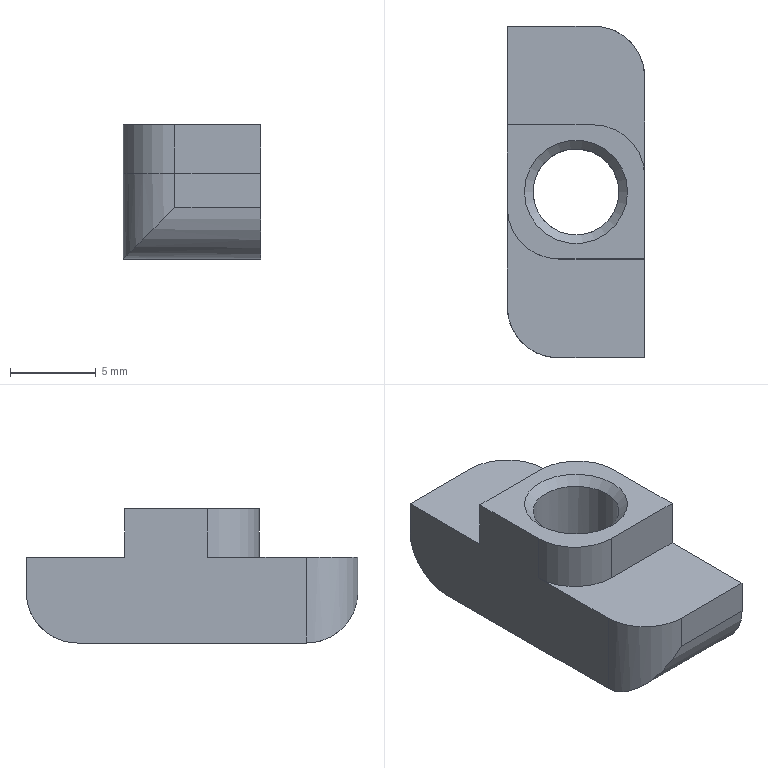Part | NX | features DATUM_CSYS 4, SKETCH 3, EXTRUDE 2, BLEND 1, HOLE PACKAGE 1, SIMPLE HOLE 1, SYMBOLIC_THREAD 1 | 1 solid | 19 faces | box 8 x 19.3 x 7.8 mm | volume 733.523 mm3 | plane 10 | cylinder 7 | cone 2 | commonest cylinder face diameters 6 x6 5 x1
STEP:
#1=CARTESIAN_POINT('',(1.,3.9,0.));
#2=VERTEX_POINT('',#1);
#3=CARTESIAN_POINT('',(-4.,3.9,0.));
#4=VERTEX_POINT('',#3);
#5=CARTESIAN_POINT('',(1.,3.9,0.));
#6=DIRECTION('',(-1.,0.,0.));
#7=VECTOR('',#6,1000.);
#8=LINE('',#5,#7);
#9=EDGE_CURVE('',#2,#4,#8,.T.);
#10=ORIENTED_EDGE('',*,*,#9,.F.);
#11=CARTESIAN_POINT('',(4.,0.9,0.));
#12=VERTEX_POINT('',#11);
#13=CARTESIAN_POINT('',(1.,0.9,0.));
#14=DIRECTION('',(0.,0.,1.));
#15=DIRECTION('',(1.,0.,0.));
#16=AXIS2_PLACEMENT_3D('',#13,#14,#15);
#17=CIRCLE('',#16,3.);
#18=EDGE_CURVE('',#12,#2,#17,.T.);
#19=ORIENTED_EDGE('',*,*,#18,.F.);
#20=CARTESIAN_POINT('',(4.,6.65,0.));
#21=VERTEX_POINT('',#20);
#22=CARTESIAN_POINT('',(4.,0.,0.));
#23=DIRECTION('',(0.,-1.,0.));
#24=VECTOR('',#23,1000.);
#25=LINE('',#22,#24);
#26=EDGE_CURVE('',#21,#12,#25,.T.);
#27=ORIENTED_EDGE('',*,*,#26,.F.);
#28=CARTESIAN_POINT('',(1.,9.65,0.));
#29=VERTEX_POINT('',#28);
#30=CARTESIAN_POINT('',(1.,6.65,0.));
#31=DIRECTION('',(0.,0.,-1.));
#32=DIRECTION('',(0.,1.,0.));
#33=AXIS2_PLACEMENT_3D('',#30,#31,#32);
#34=CIRCLE('',#33,3.);
#35=EDGE_CURVE('',#21,#29,#34,.F.);
#36=ORIENTED_EDGE('',*,*,#35,.T.);
#37=CARTESIAN_POINT('',(-4.,9.65,0.));
#38=VERTEX_POINT('',#37);
#39=CARTESIAN_POINT('',(4.,9.65,0.));
#40=DIRECTION('',(-1.,0.,0.));
#41=VECTOR('',#40,1000.);
#42=LINE('',#39,#41);
#43=EDGE_CURVE('',#29,#38,#42,.T.);
#44=ORIENTED_EDGE('',*,*,#43,.T.);
#45=CARTESIAN_POINT('',(-4.,9.65,0.));
#46=DIRECTION('',(0.,-1.,0.));
#47=VECTOR('',#46,1000.);
#48=LINE('',#45,#47);
#49=EDGE_CURVE('',#38,#4,#48,.T.);
#50=ORIENTED_EDGE('',*,*,#49,.T.);
#51=EDGE_LOOP('',(#10,#19,#27,#36,#44,#50));
#52=FACE_BOUND('',#51,.T.);
#53=CARTESIAN_POINT('',(4.,9.65,0.));
#54=DIRECTION('',(0.,0.,-1.));
#55=DIRECTION('',(0.,1.,0.));
#56=AXIS2_PLACEMENT_3D('',#53,#54,#55);
#57=PLANE('',#56);
#58=ADVANCED_FACE('',(#52),#57,.F.);
#59=CARTESIAN_POINT('',(4.,-9.65,0.));
#60=VERTEX_POINT('',#59);
#61=CARTESIAN_POINT('',(-1.,-9.65,0.));
#62=VERTEX_POINT('',#61);
#63=CARTESIAN_POINT('',(4.,-9.65,0.));
#64=DIRECTION('',(-1.,0.,0.));
#65=VECTOR('',#64,1000.);
#66=LINE('',#63,#65);
#67=EDGE_CURVE('',#60,#62,#66,.T.);
#68=ORIENTED_EDGE('',*,*,#67,.T.);
#69=CARTESIAN_POINT('',(-1.,-9.65,-2.));
#70=VERTEX_POINT('',#69);
#71=CARTESIAN_POINT('',(-1.,-9.65,0.));
#72=DIRECTION('',(0.,0.,-1.));
#73=VECTOR('',#72,1000.);
#74=LINE('',#71,#73);
#75=EDGE_CURVE('',#62,#70,#74,.T.);
#76=ORIENTED_EDGE('',*,*,#75,.T.);
#77=CARTESIAN_POINT('',(4.,-9.65,-2.));
#78=VERTEX_POINT('',#77);
#79=CARTESIAN_POINT('',(4.,-9.65,-2.));
#80=DIRECTION('',(-1.,0.,0.));
#81=VECTOR('',#80,1000.);
#82=LINE('',#79,#81);
#83=EDGE_CURVE('',#78,#70,#82,.T.);
#84=ORIENTED_EDGE('',*,*,#83,.F.);
#85=CARTESIAN_POINT('',(4.,-9.65,0.));
#86=DIRECTION('',(0.,0.,-1.));
#87=VECTOR('',#86,1000.);
#88=LINE('',#85,#87);
#89=EDGE_CURVE('',#60,#78,#88,.T.);
#90=ORIENTED_EDGE('',*,*,#89,.F.);
#91=EDGE_LOOP('',(#68,#76,#84,#90));
#92=FACE_BOUND('',#91,.T.);
#93=CARTESIAN_POINT('',(4.,-9.65,0.));
#94=DIRECTION('',(0.,1.,0.));
#95=DIRECTION('',(0.,0.,1.));
#96=AXIS2_PLACEMENT_3D('',#93,#94,#95);
#97=PLANE('',#96);
#98=ADVANCED_FACE('',(#92),#97,.F.);
#99=ORIENTED_EDGE('',*,*,#83,.T.);
#100=CARTESIAN_POINT('',(-4.,-6.65,-5.));
#101=VERTEX_POINT('',#100);
#102=CARTESIAN_POINT('',(-1.,-6.65,-2.));
#103=DIRECTION('',(0.7071,0.,-0.7071));
#104=DIRECTION('',(-0.7071,0.,-0.7071));
#105=AXIS2_PLACEMENT_3D('',#102,#103,#104);
#106=ELLIPSE('',#105,4.243,3.);
#107=EDGE_CURVE('',#70,#101,#106,.T.);
#108=ORIENTED_EDGE('',*,*,#107,.T.);
#109=CARTESIAN_POINT('',(4.,-6.65,-5.));
#110=VERTEX_POINT('',#109);
#111=CARTESIAN_POINT('',(4.,-6.65,-5.));
#112=DIRECTION('',(-1.,0.,0.));
#113=VECTOR('',#112,1000.);
#114=LINE('',#111,#113);
#115=EDGE_CURVE('',#110,#101,#114,.T.);
#116=ORIENTED_EDGE('',*,*,#115,.F.);
#117=CARTESIAN_POINT('',(4.,-6.65,-2.));
#118=DIRECTION('',(1.,0.,0.));
#119=DIRECTION('',(0.,1.,0.));
#120=AXIS2_PLACEMENT_3D('',#117,#118,#119);
#121=CIRCLE('',#120,3.);
#122=EDGE_CURVE('',#78,#110,#121,.T.);
#123=ORIENTED_EDGE('',*,*,#122,.F.);
#124=EDGE_LOOP('',(#99,#108,#116,#123));
#125=FACE_BOUND('',#124,.T.);
#126=CARTESIAN_POINT('',(4.,-6.65,-2.));
#127=DIRECTION('',(-1.,0.,0.));
#128=DIRECTION('',(0.,0.,1.));
#129=AXIS2_PLACEMENT_3D('',#126,#127,#128);
#130=CYLINDRICAL_SURFACE('',#129,3.);
#131=ADVANCED_FACE('',(#125),#130,.T.);
#132=CARTESIAN_POINT('',(0.,-3.,-5.));
#133=VERTEX_POINT('',#132);
#134=CARTESIAN_POINT('',(0.,0.,-5.));
#135=DIRECTION('',(0.,0.,1.));
#136=DIRECTION('',(0.,-1.,0.));
#137=AXIS2_PLACEMENT_3D('',#134,#135,#136);
#138=CIRCLE('',#137,3.);
#139=EDGE_CURVE('',#133,#133,#138,.T.);
#140=ORIENTED_EDGE('',*,*,#139,.T.);
#141=EDGE_LOOP('',(#140));
#142=FACE_BOUND('',#141,.T.);
#143=CARTESIAN_POINT('',(-4.,6.65,-5.));
#144=VERTEX_POINT('',#143);
#145=CARTESIAN_POINT('',(-4.,0.,-5.));
#146=DIRECTION('',(0.,1.,0.));
#147=VECTOR('',#146,1000.);
#148=LINE('',#145,#147);
#149=EDGE_CURVE('',#101,#144,#148,.T.);
#150=ORIENTED_EDGE('',*,*,#149,.T.);
#151=CARTESIAN_POINT('',(4.,6.65,-5.));
#152=VERTEX_POINT('',#151);
#153=CARTESIAN_POINT('',(4.,6.65,-5.));
#154=DIRECTION('',(-1.,0.,0.));
#155=VECTOR('',#154,1000.);
#156=LINE('',#153,#155);
#157=EDGE_CURVE('',#152,#144,#156,.T.);
#158=ORIENTED_EDGE('',*,*,#157,.F.);
#159=CARTESIAN_POINT('',(4.,-6.65,-5.));
#160=DIRECTION('',(0.,1.,0.));
#161=VECTOR('',#160,1000.);
#162=LINE('',#159,#161);
#163=EDGE_CURVE('',#110,#152,#162,.T.);
#164=ORIENTED_EDGE('',*,*,#163,.F.);
#165=ORIENTED_EDGE('',*,*,#115,.T.);
#166=EDGE_LOOP('',(#150,#158,#164,#165));
#167=FACE_BOUND('',#166,.T.);
#168=CARTESIAN_POINT('',(4.,0.,-5.));
#169=DIRECTION('',(0.,0.,1.));
#170=DIRECTION('',(0.,-1.,0.));
#171=AXIS2_PLACEMENT_3D('',#168,#169,#170);
#172=PLANE('',#171);
#173=ADVANCED_FACE('',(#142,#167),#172,.F.);
#174=CARTESIAN_POINT('',(1.,9.65,-2.));
#175=VERTEX_POINT('',#174);
#176=CARTESIAN_POINT('',(-4.,9.65,-2.));
#177=VERTEX_POINT('',#176);
#178=CARTESIAN_POINT('',(4.,9.65,-2.));
#179=DIRECTION('',(-1.,0.,0.));
#180=VECTOR('',#179,1000.);
#181=LINE('',#178,#180);
#182=EDGE_CURVE('',#175,#177,#181,.T.);
#183=ORIENTED_EDGE('',*,*,#182,.F.);
#184=CARTESIAN_POINT('',(1.,6.65,-2.));
#185=DIRECTION('',(-0.7071,0.,-0.7071));
#186=DIRECTION('',(0.7071,0.,-0.7071));
#187=AXIS2_PLACEMENT_3D('',#184,#185,#186);
#188=ELLIPSE('',#187,4.243,3.);
#189=EDGE_CURVE('',#175,#152,#188,.T.);
#190=ORIENTED_EDGE('',*,*,#189,.T.);
#191=ORIENTED_EDGE('',*,*,#157,.T.);
#192=CARTESIAN_POINT('',(-4.,6.65,-2.));
#193=DIRECTION('',(1.,0.,0.));
#194=DIRECTION('',(0.,-1.,0.));
#195=AXIS2_PLACEMENT_3D('',#192,#193,#194);
#196=CIRCLE('',#195,3.);
#197=EDGE_CURVE('',#144,#177,#196,.T.);
#198=ORIENTED_EDGE('',*,*,#197,.T.);
#199=EDGE_LOOP('',(#183,#190,#191,#198));
#200=FACE_BOUND('',#199,.T.);
#201=CARTESIAN_POINT('',(4.,6.65,-2.));
#202=DIRECTION('',(-1.,0.,0.));
#203=DIRECTION('',(0.,0.,1.));
#204=AXIS2_PLACEMENT_3D('',#201,#202,#203);
#205=CYLINDRICAL_SURFACE('',#204,3.);
#206=ADVANCED_FACE('',(#200),#205,.T.);
#207=ORIENTED_EDGE('',*,*,#43,.F.);
#208=CARTESIAN_POINT('',(1.,9.65,-2.));
#209=DIRECTION('',(0.,0.,1.));
#210=VECTOR('',#209,1000.);
#211=LINE('',#208,#210);
#212=EDGE_CURVE('',#29,#175,#211,.F.);
#213=ORIENTED_EDGE('',*,*,#212,.T.);
#214=ORIENTED_EDGE('',*,*,#182,.T.);
#215=CARTESIAN_POINT('',(-4.,9.65,-2.));
#216=DIRECTION('',(0.,0.,1.));
#217=VECTOR('',#216,1000.);
#218=LINE('',#215,#217);
#219=EDGE_CURVE('',#177,#38,#218,.T.);
#220=ORIENTED_EDGE('',*,*,#219,.T.);
#221=EDGE_LOOP('',(#207,#213,#214,#220));
#222=FACE_BOUND('',#221,.T.);
#223=CARTESIAN_POINT('',(4.,9.65,-2.));
#224=DIRECTION('',(0.,-1.,0.));
#225=DIRECTION('',(0.,0.,-1.));
#226=AXIS2_PLACEMENT_3D('',#223,#224,#225);
#227=PLANE('',#226);
#228=ADVANCED_FACE('',(#222),#227,.F.);
#229=CARTESIAN_POINT('',(-1.,-3.9,0.));
#230=VERTEX_POINT('',#229);
#231=CARTESIAN_POINT('',(4.,-3.9,0.));
#232=VERTEX_POINT('',#231);
#233=CARTESIAN_POINT('',(-1.,-3.9,0.));
#234=DIRECTION('',(1.,0.,0.));
#235=VECTOR('',#234,1000.);
#236=LINE('',#233,#235);
#237=EDGE_CURVE('',#230,#232,#236,.T.);
#238=ORIENTED_EDGE('',*,*,#237,.F.);
#239=CARTESIAN_POINT('',(-4.,-0.9,0.));
#240=VERTEX_POINT('',#239);
#241=CARTESIAN_POINT('',(-1.,-0.9,0.));
#242=DIRECTION('',(0.,0.,1.));
#243=DIRECTION('',(1.,0.,0.));
#244=AXIS2_PLACEMENT_3D('',#241,#242,#243);
#245=CIRCLE('',#244,3.);
#246=EDGE_CURVE('',#240,#230,#245,.T.);
#247=ORIENTED_EDGE('',*,*,#246,.F.);
#248=CARTESIAN_POINT('',(-4.,-6.65,0.));
#249=VERTEX_POINT('',#248);
#250=CARTESIAN_POINT('',(-4.,9.65,0.));
#251=DIRECTION('',(0.,-1.,0.));
#252=VECTOR('',#251,1000.);
#253=LINE('',#250,#252);
#254=EDGE_CURVE('',#240,#249,#253,.T.);
#255=ORIENTED_EDGE('',*,*,#254,.T.);
#256=CARTESIAN_POINT('',(-1.,-6.65,0.));
#257=DIRECTION('',(0.,0.,-1.));
#258=DIRECTION('',(0.,1.,0.));
#259=AXIS2_PLACEMENT_3D('',#256,#257,#258);
#260=CIRCLE('',#259,3.);
#261=EDGE_CURVE('',#249,#62,#260,.F.);
#262=ORIENTED_EDGE('',*,*,#261,.T.);
#263=ORIENTED_EDGE('',*,*,#67,.F.);
#264=CARTESIAN_POINT('',(4.,0.,0.));
#265=DIRECTION('',(0.,-1.,0.));
#266=VECTOR('',#265,1000.);
#267=LINE('',#264,#266);
#268=EDGE_CURVE('',#232,#60,#267,.T.);
#269=ORIENTED_EDGE('',*,*,#268,.F.);
#270=EDGE_LOOP('',(#238,#247,#255,#262,#263,#269));
#271=FACE_BOUND('',#270,.T.);
#272=CARTESIAN_POINT('',(4.,9.65,0.));
#273=DIRECTION('',(0.,0.,-1.));
#274=DIRECTION('',(0.,1.,0.));
#275=AXIS2_PLACEMENT_3D('',#272,#273,#274);
#276=PLANE('',#275);
#277=ADVANCED_FACE('',(#271),#276,.F.);
#278=ORIENTED_EDGE('',*,*,#163,.T.);
#279=CARTESIAN_POINT('',(4.,6.65,0.));
#280=DIRECTION('',(0.,0.,1.));
#281=VECTOR('',#280,1000.);
#282=LINE('',#279,#281);
#283=EDGE_CURVE('',#152,#21,#282,.T.);
#284=ORIENTED_EDGE('',*,*,#283,.T.);
#285=ORIENTED_EDGE('',*,*,#26,.T.);
#286=CARTESIAN_POINT('',(4.,0.9,2.8));
#287=VERTEX_POINT('',#286);
#288=CARTESIAN_POINT('',(4.,0.9,2.8));
#289=DIRECTION('',(0.,0.,-1.));
#290=VECTOR('',#289,1000.);
#291=LINE('',#288,#290);
#292=EDGE_CURVE('',#287,#12,#291,.T.);
#293=ORIENTED_EDGE('',*,*,#292,.F.);
#294=CARTESIAN_POINT('',(4.,-3.9,2.8));
#295=VERTEX_POINT('',#294);
#296=CARTESIAN_POINT('',(4.,-3.9,2.8));
#297=DIRECTION('',(0.,1.,0.));
#298=VECTOR('',#297,1000.);
#299=LINE('',#296,#298);
#300=EDGE_CURVE('',#295,#287,#299,.T.);
#301=ORIENTED_EDGE('',*,*,#300,.F.);
#302=CARTESIAN_POINT('',(4.,-3.9,2.8));
#303=DIRECTION('',(0.,0.,-1.));
#304=VECTOR('',#303,1000.);
#305=LINE('',#302,#304);
#306=EDGE_CURVE('',#295,#232,#305,.T.);
#307=ORIENTED_EDGE('',*,*,#306,.T.);
#308=ORIENTED_EDGE('',*,*,#268,.T.);
#309=ORIENTED_EDGE('',*,*,#89,.T.);
#310=ORIENTED_EDGE('',*,*,#122,.T.);
#311=EDGE_LOOP('',(#278,#284,#285,#293,#301,#307,#308,#309,#310));
#312=FACE_BOUND('',#311,.T.);
#313=CARTESIAN_POINT('',(4.,-6.65,-2.));
#314=DIRECTION('',(1.,0.,0.));
#315=DIRECTION('',(0.,0.,-1.));
#316=AXIS2_PLACEMENT_3D('',#313,#314,#315);
#317=PLANE('',#316);
#318=ADVANCED_FACE('',(#312),#317,.T.);
#319=ORIENTED_EDGE('',*,*,#149,.F.);
#320=CARTESIAN_POINT('',(-4.,-6.65,-2.));
#321=DIRECTION('',(0.,0.,-1.));
#322=VECTOR('',#321,1000.);
#323=LINE('',#320,#322);
#324=EDGE_CURVE('',#101,#249,#323,.F.);
#325=ORIENTED_EDGE('',*,*,#324,.T.);
#326=ORIENTED_EDGE('',*,*,#254,.F.);
#327=CARTESIAN_POINT('',(-4.,-0.9,2.8));
#328=VERTEX_POINT('',#327);
#329=CARTESIAN_POINT('',(-4.,-0.9,2.8));
#330=DIRECTION('',(0.,0.,-1.));
#331=VECTOR('',#330,1000.);
#332=LINE('',#329,#331);
#333=EDGE_CURVE('',#328,#240,#332,.T.);
#334=ORIENTED_EDGE('',*,*,#333,.F.);
#335=CARTESIAN_POINT('',(-4.,3.9,2.8));
#336=VERTEX_POINT('',#335);
#337=CARTESIAN_POINT('',(-4.,3.9,2.8));
#338=DIRECTION('',(0.,-1.,0.));
#339=VECTOR('',#338,1000.);
#340=LINE('',#337,#339);
#341=EDGE_CURVE('',#336,#328,#340,.T.);
#342=ORIENTED_EDGE('',*,*,#341,.F.);
#343=CARTESIAN_POINT('',(-4.,3.9,2.8));
#344=DIRECTION('',(0.,0.,-1.));
#345=VECTOR('',#344,1000.);
#346=LINE('',#343,#345);
#347=EDGE_CURVE('',#336,#4,#346,.T.);
#348=ORIENTED_EDGE('',*,*,#347,.T.);
#349=ORIENTED_EDGE('',*,*,#49,.F.);
#350=ORIENTED_EDGE('',*,*,#219,.F.);
#351=ORIENTED_EDGE('',*,*,#197,.F.);
#352=EDGE_LOOP('',(#319,#325,#326,#334,#342,#348,#349,#350,#351));
#353=FACE_BOUND('',#352,.T.);
#354=CARTESIAN_POINT('',(-4.,-6.65,-2.));
#355=DIRECTION('',(1.,0.,0.));
#356=DIRECTION('',(0.,0.,-1.));
#357=AXIS2_PLACEMENT_3D('',#354,#355,#356);
#358=PLANE('',#357);
#359=ADVANCED_FACE('',(#353),#358,.F.);
#360=ORIENTED_EDGE('',*,*,#261,.F.);
#361=ORIENTED_EDGE('',*,*,#324,.F.);
#362=ORIENTED_EDGE('',*,*,#107,.F.);
#363=ORIENTED_EDGE('',*,*,#75,.F.);
#364=EDGE_LOOP('',(#360,#361,#362,#363));
#365=FACE_BOUND('',#364,.T.);
#366=CARTESIAN_POINT('',(-1.,-6.65,0.));
#367=DIRECTION('',(0.,0.,-1.));
#368=DIRECTION('',(-1.,0.,0.));
#369=AXIS2_PLACEMENT_3D('',#366,#367,#368);
#370=CYLINDRICAL_SURFACE('',#369,3.);
#371=ADVANCED_FACE('',(#365),#370,.T.);
#372=ORIENTED_EDGE('',*,*,#189,.F.);
#373=ORIENTED_EDGE('',*,*,#212,.F.);
#374=ORIENTED_EDGE('',*,*,#35,.F.);
#375=ORIENTED_EDGE('',*,*,#283,.F.);
#376=EDGE_LOOP('',(#372,#373,#374,#375));
#377=FACE_BOUND('',#376,.T.);
#378=CARTESIAN_POINT('',(1.,6.65,-2.));
#379=DIRECTION('',(0.,0.,-1.));
#380=DIRECTION('',(-1.,0.,0.));
#381=AXIS2_PLACEMENT_3D('',#378,#379,#380);
#382=CYLINDRICAL_SURFACE('',#381,3.);
#383=ADVANCED_FACE('',(#377),#382,.T.);
#384=ORIENTED_EDGE('',*,*,#246,.T.);
#385=CARTESIAN_POINT('',(-1.,-3.9,2.8));
#386=VERTEX_POINT('',#385);
#387=CARTESIAN_POINT('',(-1.,-3.9,2.8));
#388=DIRECTION('',(0.,0.,-1.));
#389=VECTOR('',#388,1000.);
#390=LINE('',#387,#389);
#391=EDGE_CURVE('',#386,#230,#390,.T.);
#392=ORIENTED_EDGE('',*,*,#391,.F.);
#393=CARTESIAN_POINT('',(-1.,-0.9,2.8));
#394=DIRECTION('',(0.,0.,1.));
#395=DIRECTION('',(1.,0.,0.));
#396=AXIS2_PLACEMENT_3D('',#393,#394,#395);
#397=CIRCLE('',#396,3.);
#398=EDGE_CURVE('',#328,#386,#397,.T.);
#399=ORIENTED_EDGE('',*,*,#398,.F.);
#400=ORIENTED_EDGE('',*,*,#333,.T.);
#401=EDGE_LOOP('',(#384,#392,#399,#400));
#402=FACE_BOUND('',#401,.T.);
#403=CARTESIAN_POINT('',(-1.,-0.9,2.8));
#404=DIRECTION('',(0.,0.,-1.));
#405=DIRECTION('',(-1.,0.,0.));
#406=AXIS2_PLACEMENT_3D('',#403,#404,#405);
#407=CYLINDRICAL_SURFACE('',#406,3.);
#408=ADVANCED_FACE('',(#402),#407,.T.);
#409=ORIENTED_EDGE('',*,*,#237,.T.);
#410=ORIENTED_EDGE('',*,*,#306,.F.);
#411=CARTESIAN_POINT('',(-1.,-3.9,2.8));
#412=DIRECTION('',(1.,0.,0.));
#413=VECTOR('',#412,1000.);
#414=LINE('',#411,#413);
#415=EDGE_CURVE('',#386,#295,#414,.T.);
#416=ORIENTED_EDGE('',*,*,#415,.F.);
#417=ORIENTED_EDGE('',*,*,#391,.T.);
#418=EDGE_LOOP('',(#409,#410,#416,#417));
#419=FACE_BOUND('',#418,.T.);
#420=CARTESIAN_POINT('',(-1.,-3.9,2.8));
#421=DIRECTION('',(0.,1.,0.));
#422=DIRECTION('',(-1.,0.,0.));
#423=AXIS2_PLACEMENT_3D('',#420,#421,#422);
#424=PLANE('',#423);
#425=ADVANCED_FACE('',(#419),#424,.F.);
#426=ORIENTED_EDGE('',*,*,#18,.T.);
#427=CARTESIAN_POINT('',(1.,3.9,2.8));
#428=VERTEX_POINT('',#427);
#429=CARTESIAN_POINT('',(1.,3.9,2.8));
#430=DIRECTION('',(0.,0.,-1.));
#431=VECTOR('',#430,1000.);
#432=LINE('',#429,#431);
#433=EDGE_CURVE('',#428,#2,#432,.T.);
#434=ORIENTED_EDGE('',*,*,#433,.F.);
#435=CARTESIAN_POINT('',(1.,0.9,2.8));
#436=DIRECTION('',(0.,0.,1.));
#437=DIRECTION('',(1.,0.,0.));
#438=AXIS2_PLACEMENT_3D('',#435,#436,#437);
#439=CIRCLE('',#438,3.);
#440=EDGE_CURVE('',#287,#428,#439,.T.);
#441=ORIENTED_EDGE('',*,*,#440,.F.);
#442=ORIENTED_EDGE('',*,*,#292,.T.);
#443=EDGE_LOOP('',(#426,#434,#441,#442));
#444=FACE_BOUND('',#443,.T.);
#445=CARTESIAN_POINT('',(1.,0.9,2.8));
#446=DIRECTION('',(0.,0.,-1.));
#447=DIRECTION('',(-1.,0.,0.));
#448=AXIS2_PLACEMENT_3D('',#445,#446,#447);
#449=CYLINDRICAL_SURFACE('',#448,3.);
#450=ADVANCED_FACE('',(#444),#449,.T.);
#451=ORIENTED_EDGE('',*,*,#9,.T.);
#452=ORIENTED_EDGE('',*,*,#347,.F.);
#453=CARTESIAN_POINT('',(1.,3.9,2.8));
#454=DIRECTION('',(-1.,0.,0.));
#455=VECTOR('',#454,1000.);
#456=LINE('',#453,#455);
#457=EDGE_CURVE('',#428,#336,#456,.T.);
#458=ORIENTED_EDGE('',*,*,#457,.F.);
#459=ORIENTED_EDGE('',*,*,#433,.T.);
#460=EDGE_LOOP('',(#451,#452,#458,#459));
#461=FACE_BOUND('',#460,.T.);
#462=CARTESIAN_POINT('',(1.,3.9,2.8));
#463=DIRECTION('',(0.,-1.,0.));
#464=DIRECTION('',(1.,0.,0.));
#465=AXIS2_PLACEMENT_3D('',#462,#463,#464);
#466=PLANE('',#465);
#467=ADVANCED_FACE('',(#461),#466,.F.);
#468=CARTESIAN_POINT('',(3.,0.,2.8));
#469=VERTEX_POINT('',#468);
#470=CARTESIAN_POINT('',(0.,0.,2.8));
#471=DIRECTION('',(0.,0.,1.));
#472=DIRECTION('',(1.,0.,0.));
#473=AXIS2_PLACEMENT_3D('',#470,#471,#472);
#474=CIRCLE('',#473,3.);
#475=EDGE_CURVE('',#469,#469,#474,.F.);
#476=ORIENTED_EDGE('',*,*,#475,.T.);
#477=EDGE_LOOP('',(#476));
#478=FACE_BOUND('',#477,.T.);
#479=ORIENTED_EDGE('',*,*,#341,.T.);
#480=ORIENTED_EDGE('',*,*,#398,.T.);
#481=ORIENTED_EDGE('',*,*,#415,.T.);
#482=ORIENTED_EDGE('',*,*,#300,.T.);
#483=ORIENTED_EDGE('',*,*,#440,.T.);
#484=ORIENTED_EDGE('',*,*,#457,.T.);
#485=EDGE_LOOP('',(#479,#480,#481,#482,#483,#484));
#486=FACE_BOUND('',#485,.T.);
#487=CARTESIAN_POINT('',(-1.,-0.9,2.8));
#488=DIRECTION('',(0.,0.,1.));
#489=DIRECTION('',(1.,0.,0.));
#490=AXIS2_PLACEMENT_3D('',#487,#488,#489);
#491=PLANE('',#490);
#492=ADVANCED_FACE('',(#478,#486),#491,.T.);
#493=CARTESIAN_POINT('',(2.5,0.,-4.5));
#494=VERTEX_POINT('',#493);
#495=CARTESIAN_POINT('',(0.,0.,-4.5));
#496=DIRECTION('',(0.,0.,1.));
#497=DIRECTION('',(1.,0.,0.));
#498=AXIS2_PLACEMENT_3D('',#495,#496,#497);
#499=CIRCLE('',#498,2.5);
#500=EDGE_CURVE('',#494,#494,#499,.F.);
#501=ORIENTED_EDGE('',*,*,#500,.T.);
#502=EDGE_LOOP('',(#501));
#503=FACE_BOUND('',#502,.T.);
#504=CARTESIAN_POINT('',(2.5,0.,2.3));
#505=VERTEX_POINT('',#504);
#506=CARTESIAN_POINT('',(0.,0.,2.3));
#507=DIRECTION('',(0.,0.,1.));
#508=DIRECTION('',(1.,0.,0.));
#509=AXIS2_PLACEMENT_3D('',#506,#507,#508);
#510=CIRCLE('',#509,2.5);
#511=EDGE_CURVE('',#505,#505,#510,.T.);
#512=ORIENTED_EDGE('',*,*,#511,.T.);
#513=EDGE_LOOP('',(#512));
#514=FACE_BOUND('',#513,.T.);
#515=CARTESIAN_POINT('',(0.,0.,2.8));
#516=DIRECTION('',(0.,0.,-1.));
#517=DIRECTION('',(-1.,0.,0.));
#518=AXIS2_PLACEMENT_3D('',#515,#516,#517);
#519=CYLINDRICAL_SURFACE('',#518,2.5);
#520=ADVANCED_FACE('',(#503,#514),#519,.F.);
#521=ORIENTED_EDGE('',*,*,#511,.F.);
#522=EDGE_LOOP('',(#521));
#523=FACE_BOUND('',#522,.T.);
#524=ORIENTED_EDGE('',*,*,#475,.F.);
#525=EDGE_LOOP('',(#524));
#526=FACE_BOUND('',#525,.T.);
#527=CARTESIAN_POINT('',(0.,0.,2.8));
#528=DIRECTION('',(0.,0.,1.));
#529=DIRECTION('',(1.,0.,0.));
#530=AXIS2_PLACEMENT_3D('',#527,#528,#529);
#531=CONICAL_SURFACE('',#530,3.,0.7854);
#532=ADVANCED_FACE('',(#523,#526),#531,.F.);
#533=ORIENTED_EDGE('',*,*,#500,.F.);
#534=EDGE_LOOP('',(#533));
#535=FACE_BOUND('',#534,.T.);
#536=ORIENTED_EDGE('',*,*,#139,.F.);
#537=EDGE_LOOP('',(#536));
#538=FACE_BOUND('',#537,.T.);
#539=CARTESIAN_POINT('',(0.,0.,-5.));
#540=DIRECTION('',(0.,0.,-1.));
#541=DIRECTION('',(-1.,0.,0.));
#542=AXIS2_PLACEMENT_3D('',#539,#540,#541);
#543=CONICAL_SURFACE('',#542,3.,0.7854);
#544=ADVANCED_FACE('',(#535,#538),#543,.F.);
#545=CLOSED_SHELL('',(#58,#98,#131,#173,#206,#228,#277,#318,#359,#371,#383,#408,#425,#450,#467,#492,#520,#532,#544));
#546=MANIFOLD_SOLID_BREP('',#545);
#547=(LENGTH_UNIT()NAMED_UNIT(*)SI_UNIT(.MILLI.,.METRE.));
#548=UNCERTAINTY_MEASURE_WITH_UNIT(LENGTH_MEASURE(0.00001),#547,'','');
#549=(NAMED_UNIT(*)PLANE_ANGLE_UNIT()SI_UNIT($,.RADIAN.));
#550=(NAMED_UNIT(*)SI_UNIT($,.STERADIAN.)SOLID_ANGLE_UNIT());
#551=(GEOMETRIC_REPRESENTATION_CONTEXT(3)GLOBAL_UNCERTAINTY_ASSIGNED_CONTEXT((#548))GLOBAL_UNIT_ASSIGNED_CONTEXT((#547,#549,#550))REPRESENTATION_CONTEXT('',''));
#552=ADVANCED_BREP_SHAPE_REPRESENTATION('',(#546),#551);